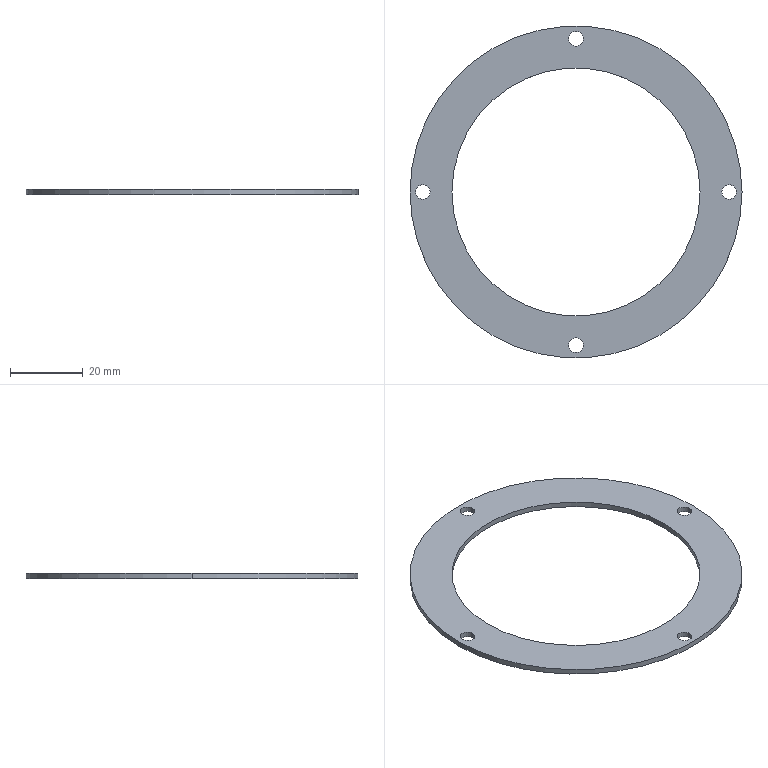Part | STEP file | 31100034--1-S0001 | 1 solid | 14 faces | box 91 x 91 x 1.5 mm | volume 4233 mm3 | cylinder 12 | plane 2 | commonest cylinder face diameters 4 x8 68 x2 91 x2
STEP:
#1=CARTESIAN_POINT('',(0.,0.,0.));
#2=DIRECTION('',(0.,0.,1.));
#3=DIRECTION('',(1.,0.,0.));
#4=AXIS2_PLACEMENT_3D('',#1,#2,#3);
#5=CARTESIAN_POINT('',(-34.,0.,-101.2));
#6=VERTEX_POINT('',#5);
#7=CARTESIAN_POINT('',(-34.,0.,-102.7));
#8=VERTEX_POINT('',#7);
#9=CARTESIAN_POINT('',(-34.,0.,-101.2));
#10=DIRECTION('',(0.,0.,-1.));
#11=VECTOR('',#10,1.);
#12=LINE('',#9,#11);
#13=CARTESIAN_POINT('',(0.,0.,-101.2));
#14=DIRECTION('',(0.,0.,-1.));
#15=DIRECTION('',(-1.,0.,0.));
#16=AXIS2_PLACEMENT_3D('',#13,#14,#15);
#17=CYLINDRICAL_SURFACE('',#16,34.);
#18=CARTESIAN_POINT('',(6.283,0.));
#19=DIRECTION('',(0.,1.));
#20=VECTOR('',#19,1.);
#21=LINE('',#18,#20);
#22=(GEOMETRIC_REPRESENTATION_CONTEXT(2)PARAMETRIC_REPRESENTATION_CONTEXT()REPRESENTATION_CONTEXT('',''));
#23=DEFINITIONAL_REPRESENTATION('',(#21),#22);
#24=PCURVE('',#17,#23);
#25=CARTESIAN_POINT('',(0.,0.,-101.2));
#26=DIRECTION('',(0.,0.,-1.));
#27=DIRECTION('',(-1.,0.,0.));
#28=AXIS2_PLACEMENT_3D('',#25,#26,#27);
#29=CYLINDRICAL_SURFACE('',#28,34.);
#30=CARTESIAN_POINT('',(0.,0.));
#31=DIRECTION('',(0.,1.));
#32=VECTOR('',#31,1.);
#33=LINE('',#30,#32);
#34=(GEOMETRIC_REPRESENTATION_CONTEXT(2)PARAMETRIC_REPRESENTATION_CONTEXT()REPRESENTATION_CONTEXT('',''));
#35=DEFINITIONAL_REPRESENTATION('',(#33),#34);
#36=PCURVE('',#29,#35);
#37=SURFACE_CURVE('',#12,(#24,#36),.PCURVE_S1.);
#38=EDGE_CURVE('',#6,#8,#37,.T.);
#39=ORIENTED_EDGE('',*,*,#38,.T.);
#40=CARTESIAN_POINT('',(34.,0.,-102.7));
#41=VERTEX_POINT('',#40);
#42=CARTESIAN_POINT('',(0.,0.,-102.7));
#43=DIRECTION('',(0.,0.,-1.));
#44=DIRECTION('',(-1.,0.,0.));
#45=AXIS2_PLACEMENT_3D('',#42,#43,#44);
#46=CIRCLE('',#45,34.);
#47=CARTESIAN_POINT('',(0.,1.5));
#48=DIRECTION('',(1.,0.));
#49=VECTOR('',#48,1.);
#50=LINE('',#47,#49);
#51=(GEOMETRIC_REPRESENTATION_CONTEXT(2)PARAMETRIC_REPRESENTATION_CONTEXT()REPRESENTATION_CONTEXT('',''));
#52=DEFINITIONAL_REPRESENTATION('',(#50),#51);
#53=PCURVE('',#17,#52);
#54=CARTESIAN_POINT('',(0.,0.,-102.7));
#55=DIRECTION('',(0.,0.,1.));
#56=DIRECTION('',(1.,0.,0.));
#57=AXIS2_PLACEMENT_3D('',#54,#55,#56);
#58=PLANE('',#57);
#59=CARTESIAN_POINT('',(-34.,0.));
#60=CARTESIAN_POINT('',(-34.,58.89));
#61=CARTESIAN_POINT('',(17.,29.445));
#62=CARTESIAN_POINT('',(68.,0.));
#63=CARTESIAN_POINT('',(17.,-29.445));
#64=CARTESIAN_POINT('',(-34.,-58.89));
#65=CARTESIAN_POINT('',(-34.,0.));
#66=(BOUNDED_CURVE()B_SPLINE_CURVE(2,(#59,#60,#61,#62,#63,#64,#65),.UNSPECIFIED.,.T.,.F.)B_SPLINE_CURVE_WITH_KNOTS((1,2,2,2,2,1),(-2.094,0.,2.094,4.189,6.283,8.378),.UNSPECIFIED.)CURVE()GEOMETRIC_REPRESENTATION_ITEM()RATIONAL_B_SPLINE_CURVE((1.,0.5,1.,0.5,1.,0.5,1.))REPRESENTATION_ITEM(''));
#67=(GEOMETRIC_REPRESENTATION_CONTEXT(2)PARAMETRIC_REPRESENTATION_CONTEXT()REPRESENTATION_CONTEXT('',''));
#68=DEFINITIONAL_REPRESENTATION('',(#66),#67);
#69=PCURVE('',#58,#68);
#70=SURFACE_CURVE('',#46,(#53,#69),.PCURVE_S1.);
#71=EDGE_CURVE('',#41,#8,#70,.T.);
#72=ORIENTED_EDGE('',*,*,#71,.F.);
#73=CARTESIAN_POINT('',(34.,0.,-101.2));
#74=VERTEX_POINT('',#73);
#75=CARTESIAN_POINT('',(34.,0.,-101.2));
#76=DIRECTION('',(0.,0.,-1.));
#77=VECTOR('',#76,1.);
#78=LINE('',#75,#77);
#79=CARTESIAN_POINT('',(3.142,0.));
#80=DIRECTION('',(0.,1.));
#81=VECTOR('',#80,1.);
#82=LINE('',#79,#81);
#83=(GEOMETRIC_REPRESENTATION_CONTEXT(2)PARAMETRIC_REPRESENTATION_CONTEXT()REPRESENTATION_CONTEXT('',''));
#84=DEFINITIONAL_REPRESENTATION('',(#82),#83);
#85=PCURVE('',#17,#84);
#86=CARTESIAN_POINT('',(3.142,0.));
#87=DIRECTION('',(0.,1.));
#88=VECTOR('',#87,1.);
#89=LINE('',#86,#88);
#90=(GEOMETRIC_REPRESENTATION_CONTEXT(2)PARAMETRIC_REPRESENTATION_CONTEXT()REPRESENTATION_CONTEXT('',''));
#91=DEFINITIONAL_REPRESENTATION('',(#89),#90);
#92=PCURVE('',#29,#91);
#93=SURFACE_CURVE('',#78,(#85,#92),.PCURVE_S1.);
#94=EDGE_CURVE('',#74,#41,#93,.T.);
#95=ORIENTED_EDGE('',*,*,#94,.F.);
#96=CARTESIAN_POINT('',(0.,0.,-101.2));
#97=DIRECTION('',(0.,0.,-1.));
#98=DIRECTION('',(-1.,0.,0.));
#99=AXIS2_PLACEMENT_3D('',#96,#97,#98);
#100=CIRCLE('',#99,34.);
#101=CARTESIAN_POINT('',(0.,0.));
#102=DIRECTION('',(1.,0.));
#103=VECTOR('',#102,1.);
#104=LINE('',#101,#103);
#105=(GEOMETRIC_REPRESENTATION_CONTEXT(2)PARAMETRIC_REPRESENTATION_CONTEXT()REPRESENTATION_CONTEXT('',''));
#106=DEFINITIONAL_REPRESENTATION('',(#104),#105);
#107=PCURVE('',#17,#106);
#108=CARTESIAN_POINT('',(0.,0.,-101.2));
#109=DIRECTION('',(0.,0.,1.));
#110=DIRECTION('',(1.,0.,0.));
#111=AXIS2_PLACEMENT_3D('',#108,#109,#110);
#112=PLANE('',#111);
#113=CARTESIAN_POINT('',(-34.,0.));
#114=CARTESIAN_POINT('',(-34.,58.89));
#115=CARTESIAN_POINT('',(17.,29.445));
#116=CARTESIAN_POINT('',(68.,0.));
#117=CARTESIAN_POINT('',(17.,-29.445));
#118=CARTESIAN_POINT('',(-34.,-58.89));
#119=CARTESIAN_POINT('',(-34.,0.));
#120=(BOUNDED_CURVE()B_SPLINE_CURVE(2,(#113,#114,#115,#116,#117,#118,#119),.UNSPECIFIED.,.T.,.F.)B_SPLINE_CURVE_WITH_KNOTS((1,2,2,2,2,1),(-2.094,0.,2.094,4.189,6.283,8.378),.UNSPECIFIED.)CURVE()GEOMETRIC_REPRESENTATION_ITEM()RATIONAL_B_SPLINE_CURVE((1.,0.5,1.,0.5,1.,0.5,1.))REPRESENTATION_ITEM(''));
#121=(GEOMETRIC_REPRESENTATION_CONTEXT(2)PARAMETRIC_REPRESENTATION_CONTEXT()REPRESENTATION_CONTEXT('',''));
#122=DEFINITIONAL_REPRESENTATION('',(#120),#121);
#123=PCURVE('',#112,#122);
#124=SURFACE_CURVE('',#100,(#107,#123),.PCURVE_S1.);
#125=EDGE_CURVE('',#74,#6,#124,.T.);
#126=ORIENTED_EDGE('',*,*,#125,.T.);
#127=EDGE_LOOP('',(#39,#72,#95,#126));
#128=FACE_BOUND('',#127,.F.);
#129=ADVANCED_FACE('',(#128),#17,.F.);
#130=CARTESIAN_POINT('',(44.,0.,-102.7));
#131=VERTEX_POINT('',#130);
#132=CARTESIAN_POINT('',(44.,0.,-101.2));
#133=VERTEX_POINT('',#132);
#134=CARTESIAN_POINT('',(44.,0.,-112.2));
#135=DIRECTION('',(0.,0.,1.));
#136=VECTOR('',#135,1.);
#137=LINE('',#134,#136);
#138=CARTESIAN_POINT('',(42.,0.,-112.2));
#139=DIRECTION('',(0.,0.,1.));
#140=DIRECTION('',(1.,0.,0.));
#141=AXIS2_PLACEMENT_3D('',#138,#139,#140);
#142=CYLINDRICAL_SURFACE('',#141,2.);
#143=CARTESIAN_POINT('',(6.283,0.));
#144=DIRECTION('',(0.,1.));
#145=VECTOR('',#144,1.);
#146=LINE('',#143,#145);
#147=(GEOMETRIC_REPRESENTATION_CONTEXT(2)PARAMETRIC_REPRESENTATION_CONTEXT()REPRESENTATION_CONTEXT('',''));
#148=DEFINITIONAL_REPRESENTATION('',(#146),#147);
#149=PCURVE('',#142,#148);
#150=CARTESIAN_POINT('',(42.,0.,-112.2));
#151=DIRECTION('',(0.,0.,1.));
#152=DIRECTION('',(1.,0.,0.));
#153=AXIS2_PLACEMENT_3D('',#150,#151,#152);
#154=CYLINDRICAL_SURFACE('',#153,2.);
#155=CARTESIAN_POINT('',(0.,0.));
#156=DIRECTION('',(0.,1.));
#157=VECTOR('',#156,1.);
#158=LINE('',#155,#157);
#159=(GEOMETRIC_REPRESENTATION_CONTEXT(2)PARAMETRIC_REPRESENTATION_CONTEXT()REPRESENTATION_CONTEXT('',''));
#160=DEFINITIONAL_REPRESENTATION('',(#158),#159);
#161=PCURVE('',#154,#160);
#162=SURFACE_CURVE('',#137,(#149,#161),.PCURVE_S1.);
#163=EDGE_CURVE('',#131,#133,#162,.T.);
#164=ORIENTED_EDGE('',*,*,#163,.T.);
#165=CARTESIAN_POINT('',(40.,0.,-101.2));
#166=VERTEX_POINT('',#165);
#167=CARTESIAN_POINT('',(42.,0.,-101.2));
#168=DIRECTION('',(0.,0.,-1.));
#169=DIRECTION('',(1.,0.,0.));
#170=AXIS2_PLACEMENT_3D('',#167,#168,#169);
#171=CIRCLE('',#170,2.);
#172=CARTESIAN_POINT('',(6.283,11.));
#173=DIRECTION('',(-1.,0.));
#174=VECTOR('',#173,1.);
#175=LINE('',#172,#174);
#176=(GEOMETRIC_REPRESENTATION_CONTEXT(2)PARAMETRIC_REPRESENTATION_CONTEXT()REPRESENTATION_CONTEXT('',''));
#177=DEFINITIONAL_REPRESENTATION('',(#175),#176);
#178=PCURVE('',#142,#177);
#179=CARTESIAN_POINT('',(44.,0.));
#180=CARTESIAN_POINT('',(44.,-3.464));
#181=CARTESIAN_POINT('',(41.,-1.732));
#182=CARTESIAN_POINT('',(38.,0.));
#183=CARTESIAN_POINT('',(41.,1.732));
#184=CARTESIAN_POINT('',(44.,3.464));
#185=CARTESIAN_POINT('',(44.,0.));
#186=(BOUNDED_CURVE()B_SPLINE_CURVE(2,(#179,#180,#181,#182,#183,#184,#185),.UNSPECIFIED.,.T.,.F.)B_SPLINE_CURVE_WITH_KNOTS((1,2,2,2,2,1),(-2.094,0.,2.094,4.189,6.283,8.378),.UNSPECIFIED.)CURVE()GEOMETRIC_REPRESENTATION_ITEM()RATIONAL_B_SPLINE_CURVE((1.,0.5,1.,0.5,1.,0.5,1.))REPRESENTATION_ITEM(''));
#187=(GEOMETRIC_REPRESENTATION_CONTEXT(2)PARAMETRIC_REPRESENTATION_CONTEXT()REPRESENTATION_CONTEXT('',''));
#188=DEFINITIONAL_REPRESENTATION('',(#186),#187);
#189=PCURVE('',#112,#188);
#190=SURFACE_CURVE('',#171,(#178,#189),.PCURVE_S1.);
#191=EDGE_CURVE('',#133,#166,#190,.T.);
#192=ORIENTED_EDGE('',*,*,#191,.T.);
#193=CARTESIAN_POINT('',(40.,0.,-102.7));
#194=VERTEX_POINT('',#193);
#195=CARTESIAN_POINT('',(40.,0.,-112.2));
#196=DIRECTION('',(0.,0.,1.));
#197=VECTOR('',#196,1.);
#198=LINE('',#195,#197);
#199=CARTESIAN_POINT('',(3.142,0.));
#200=DIRECTION('',(0.,1.));
#201=VECTOR('',#200,1.);
#202=LINE('',#199,#201);
#203=(GEOMETRIC_REPRESENTATION_CONTEXT(2)PARAMETRIC_REPRESENTATION_CONTEXT()REPRESENTATION_CONTEXT('',''));
#204=DEFINITIONAL_REPRESENTATION('',(#202),#203);
#205=PCURVE('',#142,#204);
#206=CARTESIAN_POINT('',(3.142,0.));
#207=DIRECTION('',(0.,1.));
#208=VECTOR('',#207,1.);
#209=LINE('',#206,#208);
#210=(GEOMETRIC_REPRESENTATION_CONTEXT(2)PARAMETRIC_REPRESENTATION_CONTEXT()REPRESENTATION_CONTEXT('',''));
#211=DEFINITIONAL_REPRESENTATION('',(#209),#210);
#212=PCURVE('',#154,#211);
#213=SURFACE_CURVE('',#198,(#205,#212),.PCURVE_S1.);
#214=EDGE_CURVE('',#194,#166,#213,.T.);
#215=ORIENTED_EDGE('',*,*,#214,.F.);
#216=CARTESIAN_POINT('',(42.,0.,-102.7));
#217=DIRECTION('',(0.,0.,-1.));
#218=DIRECTION('',(1.,0.,0.));
#219=AXIS2_PLACEMENT_3D('',#216,#217,#218);
#220=CIRCLE('',#219,2.);
#221=CARTESIAN_POINT('',(6.283,9.5));
#222=DIRECTION('',(-1.,0.));
#223=VECTOR('',#222,1.);
#224=LINE('',#221,#223);
#225=(GEOMETRIC_REPRESENTATION_CONTEXT(2)PARAMETRIC_REPRESENTATION_CONTEXT()REPRESENTATION_CONTEXT('',''));
#226=DEFINITIONAL_REPRESENTATION('',(#224),#225);
#227=PCURVE('',#142,#226);
#228=CARTESIAN_POINT('',(44.,0.));
#229=CARTESIAN_POINT('',(44.,-3.464));
#230=CARTESIAN_POINT('',(41.,-1.732));
#231=CARTESIAN_POINT('',(38.,0.));
#232=CARTESIAN_POINT('',(41.,1.732));
#233=CARTESIAN_POINT('',(44.,3.464));
#234=CARTESIAN_POINT('',(44.,0.));
#235=(BOUNDED_CURVE()B_SPLINE_CURVE(2,(#228,#229,#230,#231,#232,#233,#234),.UNSPECIFIED.,.T.,.F.)B_SPLINE_CURVE_WITH_KNOTS((1,2,2,2,2,1),(-2.094,0.,2.094,4.189,6.283,8.378),.UNSPECIFIED.)CURVE()GEOMETRIC_REPRESENTATION_ITEM()RATIONAL_B_SPLINE_CURVE((1.,0.5,1.,0.5,1.,0.5,1.))REPRESENTATION_ITEM(''));
#236=(GEOMETRIC_REPRESENTATION_CONTEXT(2)PARAMETRIC_REPRESENTATION_CONTEXT()REPRESENTATION_CONTEXT('',''));
#237=DEFINITIONAL_REPRESENTATION('',(#235),#236);
#238=PCURVE('',#58,#237);
#239=SURFACE_CURVE('',#220,(#227,#238),.PCURVE_S1.);
#240=EDGE_CURVE('',#131,#194,#239,.T.);
#241=ORIENTED_EDGE('',*,*,#240,.F.);
#242=EDGE_LOOP('',(#164,#192,#215,#241));
#243=FACE_BOUND('',#242,.F.);
#244=ADVANCED_FACE('',(#243),#142,.F.);
#245=CARTESIAN_POINT('',(2.,-42.,-102.7));
#246=VERTEX_POINT('',#245);
#247=CARTESIAN_POINT('',(2.,-42.,-101.2));
#248=VERTEX_POINT('',#247);
#249=CARTESIAN_POINT('',(2.,-42.,-112.2));
#250=DIRECTION('',(0.,0.,1.));
#251=VECTOR('',#250,1.);
#252=LINE('',#249,#251);
#253=CARTESIAN_POINT('',(0.,-42.,-112.2));
#254=DIRECTION('',(0.,0.,1.));
#255=DIRECTION('',(1.,0.,0.));
#256=AXIS2_PLACEMENT_3D('',#253,#254,#255);
#257=CYLINDRICAL_SURFACE('',#256,2.);
#258=CARTESIAN_POINT('',(6.283,0.));
#259=DIRECTION('',(0.,1.));
#260=VECTOR('',#259,1.);
#261=LINE('',#258,#260);
#262=(GEOMETRIC_REPRESENTATION_CONTEXT(2)PARAMETRIC_REPRESENTATION_CONTEXT()REPRESENTATION_CONTEXT('',''));
#263=DEFINITIONAL_REPRESENTATION('',(#261),#262);
#264=PCURVE('',#257,#263);
#265=CARTESIAN_POINT('',(0.,-42.,-112.2));
#266=DIRECTION('',(0.,0.,1.));
#267=DIRECTION('',(1.,0.,0.));
#268=AXIS2_PLACEMENT_3D('',#265,#266,#267);
#269=CYLINDRICAL_SURFACE('',#268,2.);
#270=CARTESIAN_POINT('',(0.,0.));
#271=DIRECTION('',(0.,1.));
#272=VECTOR('',#271,1.);
#273=LINE('',#270,#272);
#274=(GEOMETRIC_REPRESENTATION_CONTEXT(2)PARAMETRIC_REPRESENTATION_CONTEXT()REPRESENTATION_CONTEXT('',''));
#275=DEFINITIONAL_REPRESENTATION('',(#273),#274);
#276=PCURVE('',#269,#275);
#277=SURFACE_CURVE('',#252,(#264,#276),.PCURVE_S1.);
#278=EDGE_CURVE('',#246,#248,#277,.T.);
#279=ORIENTED_EDGE('',*,*,#278,.T.);
#280=CARTESIAN_POINT('',(-2.,-42.,-101.2));
#281=VERTEX_POINT('',#280);
#282=CARTESIAN_POINT('',(0.,-42.,-101.2));
#283=DIRECTION('',(0.,0.,-1.));
#284=DIRECTION('',(1.,0.,0.));
#285=AXIS2_PLACEMENT_3D('',#282,#283,#284);
#286=CIRCLE('',#285,2.);
#287=CARTESIAN_POINT('',(6.283,11.));
#288=DIRECTION('',(-1.,0.));
#289=VECTOR('',#288,1.);
#290=LINE('',#287,#289);
#291=(GEOMETRIC_REPRESENTATION_CONTEXT(2)PARAMETRIC_REPRESENTATION_CONTEXT()REPRESENTATION_CONTEXT('',''));
#292=DEFINITIONAL_REPRESENTATION('',(#290),#291);
#293=PCURVE('',#257,#292);
#294=CARTESIAN_POINT('',(2.,-42.));
#295=CARTESIAN_POINT('',(2.,-45.464));
#296=CARTESIAN_POINT('',(-1.,-43.732));
#297=CARTESIAN_POINT('',(-4.,-42.));
#298=CARTESIAN_POINT('',(-1.,-40.268));
#299=CARTESIAN_POINT('',(2.,-38.536));
#300=CARTESIAN_POINT('',(2.,-42.));
#301=(BOUNDED_CURVE()B_SPLINE_CURVE(2,(#294,#295,#296,#297,#298,#299,#300),.UNSPECIFIED.,.T.,.F.)B_SPLINE_CURVE_WITH_KNOTS((1,2,2,2,2,1),(-2.094,0.,2.094,4.189,6.283,8.378),.UNSPECIFIED.)CURVE()GEOMETRIC_REPRESENTATION_ITEM()RATIONAL_B_SPLINE_CURVE((1.,0.5,1.,0.5,1.,0.5,1.))REPRESENTATION_ITEM(''));
#302=(GEOMETRIC_REPRESENTATION_CONTEXT(2)PARAMETRIC_REPRESENTATION_CONTEXT()REPRESENTATION_CONTEXT('',''));
#303=DEFINITIONAL_REPRESENTATION('',(#301),#302);
#304=PCURVE('',#112,#303);
#305=SURFACE_CURVE('',#286,(#293,#304),.PCURVE_S1.);
#306=EDGE_CURVE('',#248,#281,#305,.T.);
#307=ORIENTED_EDGE('',*,*,#306,.T.);
#308=CARTESIAN_POINT('',(-2.,-42.,-102.7));
#309=VERTEX_POINT('',#308);
#310=CARTESIAN_POINT('',(-2.,-42.,-112.2));
#311=DIRECTION('',(0.,0.,1.));
#312=VECTOR('',#311,1.);
#313=LINE('',#310,#312);
#314=CARTESIAN_POINT('',(3.142,0.));
#315=DIRECTION('',(0.,1.));
#316=VECTOR('',#315,1.);
#317=LINE('',#314,#316);
#318=(GEOMETRIC_REPRESENTATION_CONTEXT(2)PARAMETRIC_REPRESENTATION_CONTEXT()REPRESENTATION_CONTEXT('',''));
#319=DEFINITIONAL_REPRESENTATION('',(#317),#318);
#320=PCURVE('',#257,#319);
#321=CARTESIAN_POINT('',(3.142,0.));
#322=DIRECTION('',(0.,1.));
#323=VECTOR('',#322,1.);
#324=LINE('',#321,#323);
#325=(GEOMETRIC_REPRESENTATION_CONTEXT(2)PARAMETRIC_REPRESENTATION_CONTEXT()REPRESENTATION_CONTEXT('',''));
#326=DEFINITIONAL_REPRESENTATION('',(#324),#325);
#327=PCURVE('',#269,#326);
#328=SURFACE_CURVE('',#313,(#320,#327),.PCURVE_S1.);
#329=EDGE_CURVE('',#309,#281,#328,.T.);
#330=ORIENTED_EDGE('',*,*,#329,.F.);
#331=CARTESIAN_POINT('',(0.,-42.,-102.7));
#332=DIRECTION('',(0.,0.,-1.));
#333=DIRECTION('',(1.,0.,0.));
#334=AXIS2_PLACEMENT_3D('',#331,#332,#333);
#335=CIRCLE('',#334,2.);
#336=CARTESIAN_POINT('',(6.283,9.5));
#337=DIRECTION('',(-1.,0.));
#338=VECTOR('',#337,1.);
#339=LINE('',#336,#338);
#340=(GEOMETRIC_REPRESENTATION_CONTEXT(2)PARAMETRIC_REPRESENTATION_CONTEXT()REPRESENTATION_CONTEXT('',''));
#341=DEFINITIONAL_REPRESENTATION('',(#339),#340);
#342=PCURVE('',#257,#341);
#343=CARTESIAN_POINT('',(2.,-42.));
#344=CARTESIAN_POINT('',(2.,-45.464));
#345=CARTESIAN_POINT('',(-1.,-43.732));
#346=CARTESIAN_POINT('',(-4.,-42.));
#347=CARTESIAN_POINT('',(-1.,-40.268));
#348=CARTESIAN_POINT('',(2.,-38.536));
#349=CARTESIAN_POINT('',(2.,-42.));
#350=(BOUNDED_CURVE()B_SPLINE_CURVE(2,(#343,#344,#345,#346,#347,#348,#349),.UNSPECIFIED.,.T.,.F.)B_SPLINE_CURVE_WITH_KNOTS((1,2,2,2,2,1),(-2.094,0.,2.094,4.189,6.283,8.378),.UNSPECIFIED.)CURVE()GEOMETRIC_REPRESENTATION_ITEM()RATIONAL_B_SPLINE_CURVE((1.,0.5,1.,0.5,1.,0.5,1.))REPRESENTATION_ITEM(''));
#351=(GEOMETRIC_REPRESENTATION_CONTEXT(2)PARAMETRIC_REPRESENTATION_CONTEXT()REPRESENTATION_CONTEXT('',''));
#352=DEFINITIONAL_REPRESENTATION('',(#350),#351);
#353=PCURVE('',#58,#352);
#354=SURFACE_CURVE('',#335,(#342,#353),.PCURVE_S1.);
#355=EDGE_CURVE('',#246,#309,#354,.T.);
#356=ORIENTED_EDGE('',*,*,#355,.F.);
#357=EDGE_LOOP('',(#279,#307,#330,#356));
#358=FACE_BOUND('',#357,.F.);
#359=ADVANCED_FACE('',(#358),#257,.F.);
#360=CARTESIAN_POINT('',(-40.,0.,-102.7));
#361=VERTEX_POINT('',#360);
#362=CARTESIAN_POINT('',(-40.,0.,-101.2));
#363=VERTEX_POINT('',#362);
#364=CARTESIAN_POINT('',(-40.,0.,-112.2));
#365=DIRECTION('',(0.,0.,1.));
#366=VECTOR('',#365,1.);
#367=LINE('',#364,#366);
#368=CARTESIAN_POINT('',(-42.,0.,-112.2));
#369=DIRECTION('',(0.,0.,1.));
#370=DIRECTION('',(1.,0.,0.));
#371=AXIS2_PLACEMENT_3D('',#368,#369,#370);
#372=CYLINDRICAL_SURFACE('',#371,2.);
#373=CARTESIAN_POINT('',(6.283,0.));
#374=DIRECTION('',(0.,1.));
#375=VECTOR('',#374,1.);
#376=LINE('',#373,#375);
#377=(GEOMETRIC_REPRESENTATION_CONTEXT(2)PARAMETRIC_REPRESENTATION_CONTEXT()REPRESENTATION_CONTEXT('',''));
#378=DEFINITIONAL_REPRESENTATION('',(#376),#377);
#379=PCURVE('',#372,#378);
#380=CARTESIAN_POINT('',(-42.,0.,-112.2));
#381=DIRECTION('',(0.,0.,1.));
#382=DIRECTION('',(1.,0.,0.));
#383=AXIS2_PLACEMENT_3D('',#380,#381,#382);
#384=CYLINDRICAL_SURFACE('',#383,2.);
#385=CARTESIAN_POINT('',(0.,0.));
#386=DIRECTION('',(0.,1.));
#387=VECTOR('',#386,1.);
#388=LINE('',#385,#387);
#389=(GEOMETRIC_REPRESENTATION_CONTEXT(2)PARAMETRIC_REPRESENTATION_CONTEXT()REPRESENTATION_CONTEXT('',''));
#390=DEFINITIONAL_REPRESENTATION('',(#388),#389);
#391=PCURVE('',#384,#390);
#392=SURFACE_CURVE('',#367,(#379,#391),.PCURVE_S1.);
#393=EDGE_CURVE('',#361,#363,#392,.T.);
#394=ORIENTED_EDGE('',*,*,#393,.T.);
#395=CARTESIAN_POINT('',(-44.,0.,-101.2));
#396=VERTEX_POINT('',#395);
#397=CARTESIAN_POINT('',(-42.,0.,-101.2));
#398=DIRECTION('',(0.,0.,-1.));
#399=DIRECTION('',(1.,0.,0.));
#400=AXIS2_PLACEMENT_3D('',#397,#398,#399);
#401=CIRCLE('',#400,2.);
#402=CARTESIAN_POINT('',(6.283,11.));
#403=DIRECTION('',(-1.,0.));
#404=VECTOR('',#403,1.);
#405=LINE('',#402,#404);
#406=(GEOMETRIC_REPRESENTATION_CONTEXT(2)PARAMETRIC_REPRESENTATION_CONTEXT()REPRESENTATION_CONTEXT('',''));
#407=DEFINITIONAL_REPRESENTATION('',(#405),#406);
#408=PCURVE('',#372,#407);
#409=CARTESIAN_POINT('',(-40.,0.));
#410=CARTESIAN_POINT('',(-40.,-3.464));
#411=CARTESIAN_POINT('',(-43.,-1.732));
#412=CARTESIAN_POINT('',(-46.,0.));
#413=CARTESIAN_POINT('',(-43.,1.732));
#414=CARTESIAN_POINT('',(-40.,3.464));
#415=CARTESIAN_POINT('',(-40.,0.));
#416=(BOUNDED_CURVE()B_SPLINE_CURVE(2,(#409,#410,#411,#412,#413,#414,#415),.UNSPECIFIED.,.T.,.F.)B_SPLINE_CURVE_WITH_KNOTS((1,2,2,2,2,1),(-2.094,0.,2.094,4.189,6.283,8.378),.UNSPECIFIED.)CURVE()GEOMETRIC_REPRESENTATION_ITEM()RATIONAL_B_SPLINE_CURVE((1.,0.5,1.,0.5,1.,0.5,1.))REPRESENTATION_ITEM(''));
#417=(GEOMETRIC_REPRESENTATION_CONTEXT(2)PARAMETRIC_REPRESENTATION_CONTEXT()REPRESENTATION_CONTEXT('',''));
#418=DEFINITIONAL_REPRESENTATION('',(#416),#417);
#419=PCURVE('',#112,#418);
#420=SURFACE_CURVE('',#401,(#408,#419),.PCURVE_S1.);
#421=EDGE_CURVE('',#363,#396,#420,.T.);
#422=ORIENTED_EDGE('',*,*,#421,.T.);
#423=CARTESIAN_POINT('',(-44.,0.,-102.7));
#424=VERTEX_POINT('',#423);
#425=CARTESIAN_POINT('',(-44.,0.,-112.2));
#426=DIRECTION('',(0.,0.,1.));
#427=VECTOR('',#426,1.);
#428=LINE('',#425,#427);
#429=CARTESIAN_POINT('',(3.142,0.));
#430=DIRECTION('',(0.,1.));
#431=VECTOR('',#430,1.);
#432=LINE('',#429,#431);
#433=(GEOMETRIC_REPRESENTATION_CONTEXT(2)PARAMETRIC_REPRESENTATION_CONTEXT()REPRESENTATION_CONTEXT('',''));
#434=DEFINITIONAL_REPRESENTATION('',(#432),#433);
#435=PCURVE('',#372,#434);
#436=CARTESIAN_POINT('',(3.142,0.));
#437=DIRECTION('',(0.,1.));
#438=VECTOR('',#437,1.);
#439=LINE('',#436,#438);
#440=(GEOMETRIC_REPRESENTATION_CONTEXT(2)PARAMETRIC_REPRESENTATION_CONTEXT()REPRESENTATION_CONTEXT('',''));
#441=DEFINITIONAL_REPRESENTATION('',(#439),#440);
#442=PCURVE('',#384,#441);
#443=SURFACE_CURVE('',#428,(#435,#442),.PCURVE_S1.);
#444=EDGE_CURVE('',#424,#396,#443,.T.);
#445=ORIENTED_EDGE('',*,*,#444,.F.);
#446=CARTESIAN_POINT('',(-42.,0.,-102.7));
#447=DIRECTION('',(0.,0.,-1.));
#448=DIRECTION('',(1.,0.,0.));
#449=AXIS2_PLACEMENT_3D('',#446,#447,#448);
#450=CIRCLE('',#449,2.);
#451=CARTESIAN_POINT('',(6.283,9.5));
#452=DIRECTION('',(-1.,0.));
#453=VECTOR('',#452,1.);
#454=LINE('',#451,#453);
#455=(GEOMETRIC_REPRESENTATION_CONTEXT(2)PARAMETRIC_REPRESENTATION_CONTEXT()REPRESENTATION_CONTEXT('',''));
#456=DEFINITIONAL_REPRESENTATION('',(#454),#455);
#457=PCURVE('',#372,#456);
#458=CARTESIAN_POINT('',(-40.,0.));
#459=CARTESIAN_POINT('',(-40.,-3.464));
#460=CARTESIAN_POINT('',(-43.,-1.732));
#461=CARTESIAN_POINT('',(-46.,0.));
#462=CARTESIAN_POINT('',(-43.,1.732));
#463=CARTESIAN_POINT('',(-40.,3.464));
#464=CARTESIAN_POINT('',(-40.,0.));
#465=(BOUNDED_CURVE()B_SPLINE_CURVE(2,(#458,#459,#460,#461,#462,#463,#464),.UNSPECIFIED.,.T.,.F.)B_SPLINE_CURVE_WITH_KNOTS((1,2,2,2,2,1),(-2.094,0.,2.094,4.189,6.283,8.378),.UNSPECIFIED.)CURVE()GEOMETRIC_REPRESENTATION_ITEM()RATIONAL_B_SPLINE_CURVE((1.,0.5,1.,0.5,1.,0.5,1.))REPRESENTATION_ITEM(''));
#466=(GEOMETRIC_REPRESENTATION_CONTEXT(2)PARAMETRIC_REPRESENTATION_CONTEXT()REPRESENTATION_CONTEXT('',''));
#467=DEFINITIONAL_REPRESENTATION('',(#465),#466);
#468=PCURVE('',#58,#467);
#469=SURFACE_CURVE('',#450,(#457,#468),.PCURVE_S1.);
#470=EDGE_CURVE('',#361,#424,#469,.T.);
#471=ORIENTED_EDGE('',*,*,#470,.F.);
#472=EDGE_LOOP('',(#394,#422,#445,#471));
#473=FACE_BOUND('',#472,.F.);
#474=ADVANCED_FACE('',(#473),#372,.F.);
#475=CARTESIAN_POINT('',(2.,42.,-102.7));
#476=VERTEX_POINT('',#475);
#477=CARTESIAN_POINT('',(2.,42.,-101.2));
#478=VERTEX_POINT('',#477);
#479=CARTESIAN_POINT('',(2.,42.,-112.2));
#480=DIRECTION('',(0.,0.,1.));
#481=VECTOR('',#480,1.);
#482=LINE('',#479,#481);
#483=CARTESIAN_POINT('',(0.,42.,-112.2));
#484=DIRECTION('',(0.,0.,1.));
#485=DIRECTION('',(1.,0.,0.));
#486=AXIS2_PLACEMENT_3D('',#483,#484,#485);
#487=CYLINDRICAL_SURFACE('',#486,2.);
#488=CARTESIAN_POINT('',(6.283,0.));
#489=DIRECTION('',(0.,1.));
#490=VECTOR('',#489,1.);
#491=LINE('',#488,#490);
#492=(GEOMETRIC_REPRESENTATION_CONTEXT(2)PARAMETRIC_REPRESENTATION_CONTEXT()REPRESENTATION_CONTEXT('',''));
#493=DEFINITIONAL_REPRESENTATION('',(#491),#492);
#494=PCURVE('',#487,#493);
#495=CARTESIAN_POINT('',(0.,42.,-112.2));
#496=DIRECTION('',(0.,0.,1.));
#497=DIRECTION('',(1.,0.,0.));
#498=AXIS2_PLACEMENT_3D('',#495,#496,#497);
#499=CYLINDRICAL_SURFACE('',#498,2.);
#500=CARTESIAN_POINT('',(0.,0.));
#501=DIRECTION('',(0.,1.));
#502=VECTOR('',#501,1.);
#503=LINE('',#500,#502);
#504=(GEOMETRIC_REPRESENTATION_CONTEXT(2)PARAMETRIC_REPRESENTATION_CONTEXT()REPRESENTATION_CONTEXT('',''));
#505=DEFINITIONAL_REPRESENTATION('',(#503),#504);
#506=PCURVE('',#499,#505);
#507=SURFACE_CURVE('',#482,(#494,#506),.PCURVE_S1.);
#508=EDGE_CURVE('',#476,#478,#507,.T.);
#509=ORIENTED_EDGE('',*,*,#508,.T.);
#510=CARTESIAN_POINT('',(-2.,42.,-101.2));
#511=VERTEX_POINT('',#510);
#512=CARTESIAN_POINT('',(0.,42.,-101.2));
#513=DIRECTION('',(0.,0.,-1.));
#514=DIRECTION('',(1.,0.,0.));
#515=AXIS2_PLACEMENT_3D('',#512,#513,#514);
#516=CIRCLE('',#515,2.);
#517=CARTESIAN_POINT('',(6.283,11.));
#518=DIRECTION('',(-1.,0.));
#519=VECTOR('',#518,1.);
#520=LINE('',#517,#519);
#521=(GEOMETRIC_REPRESENTATION_CONTEXT(2)PARAMETRIC_REPRESENTATION_CONTEXT()REPRESENTATION_CONTEXT('',''));
#522=DEFINITIONAL_REPRESENTATION('',(#520),#521);
#523=PCURVE('',#487,#522);
#524=CARTESIAN_POINT('',(2.,42.));
#525=CARTESIAN_POINT('',(2.,38.536));
#526=CARTESIAN_POINT('',(-1.,40.268));
#527=CARTESIAN_POINT('',(-4.,42.));
#528=CARTESIAN_POINT('',(-1.,43.732));
#529=CARTESIAN_POINT('',(2.,45.464));
#530=CARTESIAN_POINT('',(2.,42.));
#531=(BOUNDED_CURVE()B_SPLINE_CURVE(2,(#524,#525,#526,#527,#528,#529,#530),.UNSPECIFIED.,.T.,.F.)B_SPLINE_CURVE_WITH_KNOTS((1,2,2,2,2,1),(-2.094,0.,2.094,4.189,6.283,8.378),.UNSPECIFIED.)CURVE()GEOMETRIC_REPRESENTATION_ITEM()RATIONAL_B_SPLINE_CURVE((1.,0.5,1.,0.5,1.,0.5,1.))REPRESENTATION_ITEM(''));
#532=(GEOMETRIC_REPRESENTATION_CONTEXT(2)PARAMETRIC_REPRESENTATION_CONTEXT()REPRESENTATION_CONTEXT('',''));
#533=DEFINITIONAL_REPRESENTATION('',(#531),#532);
#534=PCURVE('',#112,#533);
#535=SURFACE_CURVE('',#516,(#523,#534),.PCURVE_S1.);
#536=EDGE_CURVE('',#478,#511,#535,.T.);
#537=ORIENTED_EDGE('',*,*,#536,.T.);
#538=CARTESIAN_POINT('',(-2.,42.,-102.7));
#539=VERTEX_POINT('',#538);
#540=CARTESIAN_POINT('',(-2.,42.,-112.2));
#541=DIRECTION('',(0.,0.,1.));
#542=VECTOR('',#541,1.);
#543=LINE('',#540,#542);
#544=CARTESIAN_POINT('',(3.142,0.));
#545=DIRECTION('',(0.,1.));
#546=VECTOR('',#545,1.);
#547=LINE('',#544,#546);
#548=(GEOMETRIC_REPRESENTATION_CONTEXT(2)PARAMETRIC_REPRESENTATION_CONTEXT()REPRESENTATION_CONTEXT('',''));
#549=DEFINITIONAL_REPRESENTATION('',(#547),#548);
#550=PCURVE('',#487,#549);
#551=CARTESIAN_POINT('',(3.142,0.));
#552=DIRECTION('',(0.,1.));
#553=VECTOR('',#552,1.);
#554=LINE('',#551,#553);
#555=(GEOMETRIC_REPRESENTATION_CONTEXT(2)PARAMETRIC_REPRESENTATION_CONTEXT()REPRESENTATION_CONTEXT('',''));
#556=DEFINITIONAL_REPRESENTATION('',(#554),#555);
#557=PCURVE('',#499,#556);
#558=SURFACE_CURVE('',#543,(#550,#557),.PCURVE_S1.);
#559=EDGE_CURVE('',#539,#511,#558,.T.);
#560=ORIENTED_EDGE('',*,*,#559,.F.);
#561=CARTESIAN_POINT('',(0.,42.,-102.7));
#562=DIRECTION('',(0.,0.,-1.));
#563=DIRECTION('',(1.,0.,0.));
#564=AXIS2_PLACEMENT_3D('',#561,#562,#563);
#565=CIRCLE('',#564,2.);
#566=CARTESIAN_POINT('',(6.283,9.5));
#567=DIRECTION('',(-1.,0.));
#568=VECTOR('',#567,1.);
#569=LINE('',#566,#568);
#570=(GEOMETRIC_REPRESENTATION_CONTEXT(2)PARAMETRIC_REPRESENTATION_CONTEXT()REPRESENTATION_CONTEXT('',''));
#571=DEFINITIONAL_REPRESENTATION('',(#569),#570);
#572=PCURVE('',#487,#571);
#573=CARTESIAN_POINT('',(2.,42.));
#574=CARTESIAN_POINT('',(2.,38.536));
#575=CARTESIAN_POINT('',(-1.,40.268));
#576=CARTESIAN_POINT('',(-4.,42.));
#577=CARTESIAN_POINT('',(-1.,43.732));
#578=CARTESIAN_POINT('',(2.,45.464));
#579=CARTESIAN_POINT('',(2.,42.));
#580=(BOUNDED_CURVE()B_SPLINE_CURVE(2,(#573,#574,#575,#576,#577,#578,#579),.UNSPECIFIED.,.T.,.F.)B_SPLINE_CURVE_WITH_KNOTS((1,2,2,2,2,1),(-2.094,0.,2.094,4.189,6.283,8.378),.UNSPECIFIED.)CURVE()GEOMETRIC_REPRESENTATION_ITEM()RATIONAL_B_SPLINE_CURVE((1.,0.5,1.,0.5,1.,0.5,1.))REPRESENTATION_ITEM(''));
#581=(GEOMETRIC_REPRESENTATION_CONTEXT(2)PARAMETRIC_REPRESENTATION_CONTEXT()REPRESENTATION_CONTEXT('',''));
#582=DEFINITIONAL_REPRESENTATION('',(#580),#581);
#583=PCURVE('',#58,#582);
#584=SURFACE_CURVE('',#565,(#572,#583),.PCURVE_S1.);
#585=EDGE_CURVE('',#476,#539,#584,.T.);
#586=ORIENTED_EDGE('',*,*,#585,.F.);
#587=EDGE_LOOP('',(#509,#537,#560,#586));
#588=FACE_BOUND('',#587,.F.);
#589=ADVANCED_FACE('',(#588),#487,.F.);
#590=CARTESIAN_POINT('',(-45.5,0.,-101.2));
#591=VERTEX_POINT('',#590);
#592=CARTESIAN_POINT('',(45.5,0.,-101.2));
#593=VERTEX_POINT('',#592);
#594=CARTESIAN_POINT('',(0.,0.,-101.2));
#595=DIRECTION('',(0.,0.,-1.));
#596=DIRECTION('',(-1.,0.,0.));
#597=AXIS2_PLACEMENT_3D('',#594,#595,#596);
#598=CIRCLE('',#597,45.5);
#599=CARTESIAN_POINT('',(0.,0.,-101.2));
#600=DIRECTION('',(0.,0.,-1.));
#601=DIRECTION('',(-1.,0.,0.));
#602=AXIS2_PLACEMENT_3D('',#599,#600,#601);
#603=CYLINDRICAL_SURFACE('',#602,45.5);
#604=CARTESIAN_POINT('',(0.,0.));
#605=DIRECTION('',(1.,0.));
#606=VECTOR('',#605,1.);
#607=LINE('',#604,#606);
#608=(GEOMETRIC_REPRESENTATION_CONTEXT(2)PARAMETRIC_REPRESENTATION_CONTEXT()REPRESENTATION_CONTEXT('',''));
#609=DEFINITIONAL_REPRESENTATION('',(#607),#608);
#610=PCURVE('',#603,#609);
#611=CARTESIAN_POINT('',(-45.5,0.));
#612=CARTESIAN_POINT('',(-45.5,78.808));
#613=CARTESIAN_POINT('',(22.75,39.404));
#614=CARTESIAN_POINT('',(91.,0.));
#615=CARTESIAN_POINT('',(22.75,-39.404));
#616=CARTESIAN_POINT('',(-45.5,-78.808));
#617=CARTESIAN_POINT('',(-45.5,0.));
#618=(BOUNDED_CURVE()B_SPLINE_CURVE(2,(#611,#612,#613,#614,#615,#616,#617),.UNSPECIFIED.,.T.,.F.)B_SPLINE_CURVE_WITH_KNOTS((1,2,2,2,2,1),(-2.094,0.,2.094,4.189,6.283,8.378),.UNSPECIFIED.)CURVE()GEOMETRIC_REPRESENTATION_ITEM()RATIONAL_B_SPLINE_CURVE((1.,0.5,1.,0.5,1.,0.5,1.))REPRESENTATION_ITEM(''));
#619=(GEOMETRIC_REPRESENTATION_CONTEXT(2)PARAMETRIC_REPRESENTATION_CONTEXT()REPRESENTATION_CONTEXT('',''));
#620=DEFINITIONAL_REPRESENTATION('',(#618),#619);
#621=PCURVE('',#112,#620);
#622=SURFACE_CURVE('',#598,(#610,#621),.PCURVE_S1.);
#623=EDGE_CURVE('',#591,#593,#622,.T.);
#624=ORIENTED_EDGE('',*,*,#623,.T.);
#625=CARTESIAN_POINT('',(45.5,0.,-102.7));
#626=VERTEX_POINT('',#625);
#627=CARTESIAN_POINT('',(45.5,0.,-101.2));
#628=DIRECTION('',(0.,0.,-1.));
#629=VECTOR('',#628,1.);
#630=LINE('',#627,#629);
#631=CARTESIAN_POINT('',(3.142,0.));
#632=DIRECTION('',(0.,1.));
#633=VECTOR('',#632,1.);
#634=LINE('',#631,#633);
#635=(GEOMETRIC_REPRESENTATION_CONTEXT(2)PARAMETRIC_REPRESENTATION_CONTEXT()REPRESENTATION_CONTEXT('',''));
#636=DEFINITIONAL_REPRESENTATION('',(#634),#635);
#637=PCURVE('',#603,#636);
#638=CARTESIAN_POINT('',(0.,0.,-101.2));
#639=DIRECTION('',(0.,0.,-1.));
#640=DIRECTION('',(-1.,0.,0.));
#641=AXIS2_PLACEMENT_3D('',#638,#639,#640);
#642=CYLINDRICAL_SURFACE('',#641,45.5);
#643=CARTESIAN_POINT('',(3.142,0.));
#644=DIRECTION('',(0.,1.));
#645=VECTOR('',#644,1.);
#646=LINE('',#643,#645);
#647=(GEOMETRIC_REPRESENTATION_CONTEXT(2)PARAMETRIC_REPRESENTATION_CONTEXT()REPRESENTATION_CONTEXT('',''));
#648=DEFINITIONAL_REPRESENTATION('',(#646),#647);
#649=PCURVE('',#642,#648);
#650=SURFACE_CURVE('',#630,(#637,#649),.PCURVE_S1.);
#651=EDGE_CURVE('',#593,#626,#650,.T.);
#652=ORIENTED_EDGE('',*,*,#651,.T.);
#653=CARTESIAN_POINT('',(-45.5,0.,-102.7));
#654=VERTEX_POINT('',#653);
#655=CARTESIAN_POINT('',(0.,0.,-102.7));
#656=DIRECTION('',(0.,0.,1.));
#657=DIRECTION('',(-1.,0.,0.));
#658=AXIS2_PLACEMENT_3D('',#655,#656,#657);
#659=CIRCLE('',#658,45.5);
#660=CARTESIAN_POINT('',(6.283,1.5));
#661=DIRECTION('',(-1.,0.));
#662=VECTOR('',#661,1.);
#663=LINE('',#660,#662);
#664=(GEOMETRIC_REPRESENTATION_CONTEXT(2)PARAMETRIC_REPRESENTATION_CONTEXT()REPRESENTATION_CONTEXT('',''));
#665=DEFINITIONAL_REPRESENTATION('',(#663),#664);
#666=PCURVE('',#603,#665);
#667=CARTESIAN_POINT('',(0.,0.));
#668=DIRECTION('',(-1.,0.));
#669=AXIS2_PLACEMENT_2D('',#667,#668);
#670=CIRCLE('',#669,45.5);
#671=(GEOMETRIC_REPRESENTATION_CONTEXT(2)PARAMETRIC_REPRESENTATION_CONTEXT()REPRESENTATION_CONTEXT('',''));
#672=DEFINITIONAL_REPRESENTATION('',(#670),#671);
#673=PCURVE('',#58,#672);
#674=SURFACE_CURVE('',#659,(#666,#673),.PCURVE_S1.);
#675=EDGE_CURVE('',#626,#654,#674,.T.);
#676=ORIENTED_EDGE('',*,*,#675,.T.);
#677=CARTESIAN_POINT('',(-45.5,0.,-101.2));
#678=DIRECTION('',(0.,0.,-1.));
#679=VECTOR('',#678,1.);
#680=LINE('',#677,#679);
#681=CARTESIAN_POINT('',(0.,0.));
#682=DIRECTION('',(0.,1.));
#683=VECTOR('',#682,1.);
#684=LINE('',#681,#683);
#685=(GEOMETRIC_REPRESENTATION_CONTEXT(2)PARAMETRIC_REPRESENTATION_CONTEXT()REPRESENTATION_CONTEXT('',''));
#686=DEFINITIONAL_REPRESENTATION('',(#684),#685);
#687=PCURVE('',#603,#686);
#688=CARTESIAN_POINT('',(6.283,0.));
#689=DIRECTION('',(0.,1.));
#690=VECTOR('',#689,1.);
#691=LINE('',#688,#690);
#692=(GEOMETRIC_REPRESENTATION_CONTEXT(2)PARAMETRIC_REPRESENTATION_CONTEXT()REPRESENTATION_CONTEXT('',''));
#693=DEFINITIONAL_REPRESENTATION('',(#691),#692);
#694=PCURVE('',#642,#693);
#695=SURFACE_CURVE('',#680,(#687,#694),.PCURVE_S1.);
#696=EDGE_CURVE('',#591,#654,#695,.T.);
#697=ORIENTED_EDGE('',*,*,#696,.F.);
#698=EDGE_LOOP('',(#624,#652,#676,#697));
#699=FACE_BOUND('',#698,.T.);
#700=ADVANCED_FACE('',(#699),#603,.T.);
#701=CARTESIAN_POINT('',(0.,0.,-102.7));
#702=DIRECTION('',(0.,0.,-1.));
#703=DIRECTION('',(-1.,0.,0.));
#704=AXIS2_PLACEMENT_3D('',#701,#702,#703);
#705=CIRCLE('',#704,34.);
#706=CARTESIAN_POINT('',(-34.,0.));
#707=CARTESIAN_POINT('',(-34.,58.89));
#708=CARTESIAN_POINT('',(17.,29.445));
#709=CARTESIAN_POINT('',(68.,0.));
#710=CARTESIAN_POINT('',(17.,-29.445));
#711=CARTESIAN_POINT('',(-34.,-58.89));
#712=CARTESIAN_POINT('',(-34.,0.));
#713=(BOUNDED_CURVE()B_SPLINE_CURVE(2,(#706,#707,#708,#709,#710,#711,#712),.UNSPECIFIED.,.T.,.F.)B_SPLINE_CURVE_WITH_KNOTS((1,2,2,2,2,1),(-2.094,0.,2.094,4.189,6.283,8.378),.UNSPECIFIED.)CURVE()GEOMETRIC_REPRESENTATION_ITEM()RATIONAL_B_SPLINE_CURVE((1.,0.5,1.,0.5,1.,0.5,1.))REPRESENTATION_ITEM(''));
#714=(GEOMETRIC_REPRESENTATION_CONTEXT(2)PARAMETRIC_REPRESENTATION_CONTEXT()REPRESENTATION_CONTEXT('',''));
#715=DEFINITIONAL_REPRESENTATION('',(#713),#714);
#716=PCURVE('',#58,#715);
#717=CARTESIAN_POINT('',(0.,1.5));
#718=DIRECTION('',(1.,0.));
#719=VECTOR('',#718,1.);
#720=LINE('',#717,#719);
#721=(GEOMETRIC_REPRESENTATION_CONTEXT(2)PARAMETRIC_REPRESENTATION_CONTEXT()REPRESENTATION_CONTEXT('',''));
#722=DEFINITIONAL_REPRESENTATION('',(#720),#721);
#723=PCURVE('',#29,#722);
#724=SURFACE_CURVE('',#705,(#716,#723),.PCURVE_S1.);
#725=EDGE_CURVE('',#8,#41,#724,.T.);
#726=ORIENTED_EDGE('',*,*,#725,.F.);
#727=ORIENTED_EDGE('',*,*,#71,.F.);
#728=EDGE_LOOP('',(#726,#727));
#729=FACE_BOUND('',#728,.T.);
#730=ORIENTED_EDGE('',*,*,#240,.F.);
#731=CARTESIAN_POINT('',(42.,0.,-102.7));
#732=DIRECTION('',(0.,0.,-1.));
#733=DIRECTION('',(1.,0.,0.));
#734=AXIS2_PLACEMENT_3D('',#731,#732,#733);
#735=CIRCLE('',#734,2.);
#736=CARTESIAN_POINT('',(44.,0.));
#737=CARTESIAN_POINT('',(44.,-3.464));
#738=CARTESIAN_POINT('',(41.,-1.732));
#739=CARTESIAN_POINT('',(38.,0.));
#740=CARTESIAN_POINT('',(41.,1.732));
#741=CARTESIAN_POINT('',(44.,3.464));
#742=CARTESIAN_POINT('',(44.,0.));
#743=(BOUNDED_CURVE()B_SPLINE_CURVE(2,(#736,#737,#738,#739,#740,#741,#742),.UNSPECIFIED.,.T.,.F.)B_SPLINE_CURVE_WITH_KNOTS((1,2,2,2,2,1),(-2.094,0.,2.094,4.189,6.283,8.378),.UNSPECIFIED.)CURVE()GEOMETRIC_REPRESENTATION_ITEM()RATIONAL_B_SPLINE_CURVE((1.,0.5,1.,0.5,1.,0.5,1.))REPRESENTATION_ITEM(''));
#744=(GEOMETRIC_REPRESENTATION_CONTEXT(2)PARAMETRIC_REPRESENTATION_CONTEXT()REPRESENTATION_CONTEXT('',''));
#745=DEFINITIONAL_REPRESENTATION('',(#743),#744);
#746=PCURVE('',#58,#745);
#747=CARTESIAN_POINT('',(6.283,9.5));
#748=DIRECTION('',(-1.,0.));
#749=VECTOR('',#748,1.);
#750=LINE('',#747,#749);
#751=(GEOMETRIC_REPRESENTATION_CONTEXT(2)PARAMETRIC_REPRESENTATION_CONTEXT()REPRESENTATION_CONTEXT('',''));
#752=DEFINITIONAL_REPRESENTATION('',(#750),#751);
#753=PCURVE('',#154,#752);
#754=SURFACE_CURVE('',#735,(#746,#753),.PCURVE_S1.);
#755=EDGE_CURVE('',#194,#131,#754,.T.);
#756=ORIENTED_EDGE('',*,*,#755,.F.);
#757=EDGE_LOOP('',(#730,#756));
#758=FACE_BOUND('',#757,.T.);
#759=ORIENTED_EDGE('',*,*,#355,.F.);
#760=CARTESIAN_POINT('',(0.,-42.,-102.7));
#761=DIRECTION('',(0.,0.,-1.));
#762=DIRECTION('',(1.,0.,0.));
#763=AXIS2_PLACEMENT_3D('',#760,#761,#762);
#764=CIRCLE('',#763,2.);
#765=CARTESIAN_POINT('',(2.,-42.));
#766=CARTESIAN_POINT('',(2.,-45.464));
#767=CARTESIAN_POINT('',(-1.,-43.732));
#768=CARTESIAN_POINT('',(-4.,-42.));
#769=CARTESIAN_POINT('',(-1.,-40.268));
#770=CARTESIAN_POINT('',(2.,-38.536));
#771=CARTESIAN_POINT('',(2.,-42.));
#772=(BOUNDED_CURVE()B_SPLINE_CURVE(2,(#765,#766,#767,#768,#769,#770,#771),.UNSPECIFIED.,.T.,.F.)B_SPLINE_CURVE_WITH_KNOTS((1,2,2,2,2,1),(-2.094,0.,2.094,4.189,6.283,8.378),.UNSPECIFIED.)CURVE()GEOMETRIC_REPRESENTATION_ITEM()RATIONAL_B_SPLINE_CURVE((1.,0.5,1.,0.5,1.,0.5,1.))REPRESENTATION_ITEM(''));
#773=(GEOMETRIC_REPRESENTATION_CONTEXT(2)PARAMETRIC_REPRESENTATION_CONTEXT()REPRESENTATION_CONTEXT('',''));
#774=DEFINITIONAL_REPRESENTATION('',(#772),#773);
#775=PCURVE('',#58,#774);
#776=CARTESIAN_POINT('',(6.283,9.5));
#777=DIRECTION('',(-1.,0.));
#778=VECTOR('',#777,1.);
#779=LINE('',#776,#778);
#780=(GEOMETRIC_REPRESENTATION_CONTEXT(2)PARAMETRIC_REPRESENTATION_CONTEXT()REPRESENTATION_CONTEXT('',''));
#781=DEFINITIONAL_REPRESENTATION('',(#779),#780);
#782=PCURVE('',#269,#781);
#783=SURFACE_CURVE('',#764,(#775,#782),.PCURVE_S1.);
#784=EDGE_CURVE('',#309,#246,#783,.T.);
#785=ORIENTED_EDGE('',*,*,#784,.F.);
#786=EDGE_LOOP('',(#759,#785));
#787=FACE_BOUND('',#786,.T.);
#788=ORIENTED_EDGE('',*,*,#470,.F.);
#789=CARTESIAN_POINT('',(-42.,0.,-102.7));
#790=DIRECTION('',(0.,0.,-1.));
#791=DIRECTION('',(1.,0.,0.));
#792=AXIS2_PLACEMENT_3D('',#789,#790,#791);
#793=CIRCLE('',#792,2.);
#794=CARTESIAN_POINT('',(-40.,0.));
#795=CARTESIAN_POINT('',(-40.,-3.464));
#796=CARTESIAN_POINT('',(-43.,-1.732));
#797=CARTESIAN_POINT('',(-46.,0.));
#798=CARTESIAN_POINT('',(-43.,1.732));
#799=CARTESIAN_POINT('',(-40.,3.464));
#800=CARTESIAN_POINT('',(-40.,0.));
#801=(BOUNDED_CURVE()B_SPLINE_CURVE(2,(#794,#795,#796,#797,#798,#799,#800),.UNSPECIFIED.,.T.,.F.)B_SPLINE_CURVE_WITH_KNOTS((1,2,2,2,2,1),(-2.094,0.,2.094,4.189,6.283,8.378),.UNSPECIFIED.)CURVE()GEOMETRIC_REPRESENTATION_ITEM()RATIONAL_B_SPLINE_CURVE((1.,0.5,1.,0.5,1.,0.5,1.))REPRESENTATION_ITEM(''));
#802=(GEOMETRIC_REPRESENTATION_CONTEXT(2)PARAMETRIC_REPRESENTATION_CONTEXT()REPRESENTATION_CONTEXT('',''));
#803=DEFINITIONAL_REPRESENTATION('',(#801),#802);
#804=PCURVE('',#58,#803);
#805=CARTESIAN_POINT('',(6.283,9.5));
#806=DIRECTION('',(-1.,0.));
#807=VECTOR('',#806,1.);
#808=LINE('',#805,#807);
#809=(GEOMETRIC_REPRESENTATION_CONTEXT(2)PARAMETRIC_REPRESENTATION_CONTEXT()REPRESENTATION_CONTEXT('',''));
#810=DEFINITIONAL_REPRESENTATION('',(#808),#809);
#811=PCURVE('',#384,#810);
#812=SURFACE_CURVE('',#793,(#804,#811),.PCURVE_S1.);
#813=EDGE_CURVE('',#424,#361,#812,.T.);
#814=ORIENTED_EDGE('',*,*,#813,.F.);
#815=EDGE_LOOP('',(#788,#814));
#816=FACE_BOUND('',#815,.T.);
#817=ORIENTED_EDGE('',*,*,#585,.F.);
#818=CARTESIAN_POINT('',(0.,42.,-102.7));
#819=DIRECTION('',(0.,0.,-1.));
#820=DIRECTION('',(1.,0.,0.));
#821=AXIS2_PLACEMENT_3D('',#818,#819,#820);
#822=CIRCLE('',#821,2.);
#823=CARTESIAN_POINT('',(2.,42.));
#824=CARTESIAN_POINT('',(2.,38.536));
#825=CARTESIAN_POINT('',(-1.,40.268));
#826=CARTESIAN_POINT('',(-4.,42.));
#827=CARTESIAN_POINT('',(-1.,43.732));
#828=CARTESIAN_POINT('',(2.,45.464));
#829=CARTESIAN_POINT('',(2.,42.));
#830=(BOUNDED_CURVE()B_SPLINE_CURVE(2,(#823,#824,#825,#826,#827,#828,#829),.UNSPECIFIED.,.T.,.F.)B_SPLINE_CURVE_WITH_KNOTS((1,2,2,2,2,1),(-2.094,0.,2.094,4.189,6.283,8.378),.UNSPECIFIED.)CURVE()GEOMETRIC_REPRESENTATION_ITEM()RATIONAL_B_SPLINE_CURVE((1.,0.5,1.,0.5,1.,0.5,1.))REPRESENTATION_ITEM(''));
#831=(GEOMETRIC_REPRESENTATION_CONTEXT(2)PARAMETRIC_REPRESENTATION_CONTEXT()REPRESENTATION_CONTEXT('',''));
#832=DEFINITIONAL_REPRESENTATION('',(#830),#831);
#833=PCURVE('',#58,#832);
#834=CARTESIAN_POINT('',(6.283,9.5));
#835=DIRECTION('',(-1.,0.));
#836=VECTOR('',#835,1.);
#837=LINE('',#834,#836);
#838=(GEOMETRIC_REPRESENTATION_CONTEXT(2)PARAMETRIC_REPRESENTATION_CONTEXT()REPRESENTATION_CONTEXT('',''));
#839=DEFINITIONAL_REPRESENTATION('',(#837),#838);
#840=PCURVE('',#499,#839);
#841=SURFACE_CURVE('',#822,(#833,#840),.PCURVE_S1.);
#842=EDGE_CURVE('',#539,#476,#841,.T.);
#843=ORIENTED_EDGE('',*,*,#842,.F.);
#844=EDGE_LOOP('',(#817,#843));
#845=FACE_BOUND('',#844,.T.);
#846=CARTESIAN_POINT('',(0.,0.,-102.7));
#847=DIRECTION('',(0.,0.,1.));
#848=DIRECTION('',(-1.,0.,0.));
#849=AXIS2_PLACEMENT_3D('',#846,#847,#848);
#850=CIRCLE('',#849,45.5);
#851=CARTESIAN_POINT('',(0.,0.));
#852=DIRECTION('',(-1.,0.));
#853=AXIS2_PLACEMENT_2D('',#851,#852);
#854=CIRCLE('',#853,45.5);
#855=(GEOMETRIC_REPRESENTATION_CONTEXT(2)PARAMETRIC_REPRESENTATION_CONTEXT()REPRESENTATION_CONTEXT('',''));
#856=DEFINITIONAL_REPRESENTATION('',(#854),#855);
#857=PCURVE('',#58,#856);
#858=CARTESIAN_POINT('',(6.283,1.5));
#859=DIRECTION('',(-1.,0.));
#860=VECTOR('',#859,1.);
#861=LINE('',#858,#860);
#862=(GEOMETRIC_REPRESENTATION_CONTEXT(2)PARAMETRIC_REPRESENTATION_CONTEXT()REPRESENTATION_CONTEXT('',''));
#863=DEFINITIONAL_REPRESENTATION('',(#861),#862);
#864=PCURVE('',#642,#863);
#865=SURFACE_CURVE('',#850,(#857,#864),.PCURVE_S1.);
#866=EDGE_CURVE('',#654,#626,#865,.T.);
#867=ORIENTED_EDGE('',*,*,#866,.F.);
#868=ORIENTED_EDGE('',*,*,#675,.F.);
#869=EDGE_LOOP('',(#867,#868));
#870=FACE_BOUND('',#869,.T.);
#871=ADVANCED_FACE('',(#729,#758,#787,#816,#845,#870),#58,.F.);
#872=ORIENTED_EDGE('',*,*,#725,.F.);
#873=ORIENTED_EDGE('',*,*,#38,.F.);
#874=CARTESIAN_POINT('',(0.,0.,-101.2));
#875=DIRECTION('',(0.,0.,-1.));
#876=DIRECTION('',(-1.,0.,0.));
#877=AXIS2_PLACEMENT_3D('',#874,#875,#876);
#878=CIRCLE('',#877,34.);
#879=CARTESIAN_POINT('',(0.,0.));
#880=DIRECTION('',(1.,0.));
#881=VECTOR('',#880,1.);
#882=LINE('',#879,#881);
#883=(GEOMETRIC_REPRESENTATION_CONTEXT(2)PARAMETRIC_REPRESENTATION_CONTEXT()REPRESENTATION_CONTEXT('',''));
#884=DEFINITIONAL_REPRESENTATION('',(#882),#883);
#885=PCURVE('',#29,#884);
#886=CARTESIAN_POINT('',(-34.,0.));
#887=CARTESIAN_POINT('',(-34.,58.89));
#888=CARTESIAN_POINT('',(17.,29.445));
#889=CARTESIAN_POINT('',(68.,0.));
#890=CARTESIAN_POINT('',(17.,-29.445));
#891=CARTESIAN_POINT('',(-34.,-58.89));
#892=CARTESIAN_POINT('',(-34.,0.));
#893=(BOUNDED_CURVE()B_SPLINE_CURVE(2,(#886,#887,#888,#889,#890,#891,#892),.UNSPECIFIED.,.T.,.F.)B_SPLINE_CURVE_WITH_KNOTS((1,2,2,2,2,1),(-2.094,0.,2.094,4.189,6.283,8.378),.UNSPECIFIED.)CURVE()GEOMETRIC_REPRESENTATION_ITEM()RATIONAL_B_SPLINE_CURVE((1.,0.5,1.,0.5,1.,0.5,1.))REPRESENTATION_ITEM(''));
#894=(GEOMETRIC_REPRESENTATION_CONTEXT(2)PARAMETRIC_REPRESENTATION_CONTEXT()REPRESENTATION_CONTEXT('',''));
#895=DEFINITIONAL_REPRESENTATION('',(#893),#894);
#896=PCURVE('',#112,#895);
#897=SURFACE_CURVE('',#878,(#885,#896),.PCURVE_S1.);
#898=EDGE_CURVE('',#6,#74,#897,.T.);
#899=ORIENTED_EDGE('',*,*,#898,.T.);
#900=ORIENTED_EDGE('',*,*,#94,.T.);
#901=EDGE_LOOP('',(#872,#873,#899,#900));
#902=FACE_BOUND('',#901,.F.);
#903=ADVANCED_FACE('',(#902),#29,.F.);
#904=CARTESIAN_POINT('',(42.,0.,-101.2));
#905=DIRECTION('',(0.,0.,-1.));
#906=DIRECTION('',(1.,0.,0.));
#907=AXIS2_PLACEMENT_3D('',#904,#905,#906);
#908=CIRCLE('',#907,2.);
#909=CARTESIAN_POINT('',(6.283,11.));
#910=DIRECTION('',(-1.,0.));
#911=VECTOR('',#910,1.);
#912=LINE('',#909,#911);
#913=(GEOMETRIC_REPRESENTATION_CONTEXT(2)PARAMETRIC_REPRESENTATION_CONTEXT()REPRESENTATION_CONTEXT('',''));
#914=DEFINITIONAL_REPRESENTATION('',(#912),#913);
#915=PCURVE('',#154,#914);
#916=CARTESIAN_POINT('',(44.,0.));
#917=CARTESIAN_POINT('',(44.,-3.464));
#918=CARTESIAN_POINT('',(41.,-1.732));
#919=CARTESIAN_POINT('',(38.,0.));
#920=CARTESIAN_POINT('',(41.,1.732));
#921=CARTESIAN_POINT('',(44.,3.464));
#922=CARTESIAN_POINT('',(44.,0.));
#923=(BOUNDED_CURVE()B_SPLINE_CURVE(2,(#916,#917,#918,#919,#920,#921,#922),.UNSPECIFIED.,.T.,.F.)B_SPLINE_CURVE_WITH_KNOTS((1,2,2,2,2,1),(-2.094,0.,2.094,4.189,6.283,8.378),.UNSPECIFIED.)CURVE()GEOMETRIC_REPRESENTATION_ITEM()RATIONAL_B_SPLINE_CURVE((1.,0.5,1.,0.5,1.,0.5,1.))REPRESENTATION_ITEM(''));
#924=(GEOMETRIC_REPRESENTATION_CONTEXT(2)PARAMETRIC_REPRESENTATION_CONTEXT()REPRESENTATION_CONTEXT('',''));
#925=DEFINITIONAL_REPRESENTATION('',(#923),#924);
#926=PCURVE('',#112,#925);
#927=SURFACE_CURVE('',#908,(#915,#926),.PCURVE_S1.);
#928=EDGE_CURVE('',#166,#133,#927,.T.);
#929=ORIENTED_EDGE('',*,*,#928,.T.);
#930=ORIENTED_EDGE('',*,*,#163,.F.);
#931=ORIENTED_EDGE('',*,*,#755,.F.);
#932=ORIENTED_EDGE('',*,*,#214,.T.);
#933=EDGE_LOOP('',(#929,#930,#931,#932));
#934=FACE_BOUND('',#933,.F.);
#935=ADVANCED_FACE('',(#934),#154,.F.);
#936=CARTESIAN_POINT('',(0.,-42.,-101.2));
#937=DIRECTION('',(0.,0.,-1.));
#938=DIRECTION('',(1.,0.,0.));
#939=AXIS2_PLACEMENT_3D('',#936,#937,#938);
#940=CIRCLE('',#939,2.);
#941=CARTESIAN_POINT('',(6.283,11.));
#942=DIRECTION('',(-1.,0.));
#943=VECTOR('',#942,1.);
#944=LINE('',#941,#943);
#945=(GEOMETRIC_REPRESENTATION_CONTEXT(2)PARAMETRIC_REPRESENTATION_CONTEXT()REPRESENTATION_CONTEXT('',''));
#946=DEFINITIONAL_REPRESENTATION('',(#944),#945);
#947=PCURVE('',#269,#946);
#948=CARTESIAN_POINT('',(2.,-42.));
#949=CARTESIAN_POINT('',(2.,-45.464));
#950=CARTESIAN_POINT('',(-1.,-43.732));
#951=CARTESIAN_POINT('',(-4.,-42.));
#952=CARTESIAN_POINT('',(-1.,-40.268));
#953=CARTESIAN_POINT('',(2.,-38.536));
#954=CARTESIAN_POINT('',(2.,-42.));
#955=(BOUNDED_CURVE()B_SPLINE_CURVE(2,(#948,#949,#950,#951,#952,#953,#954),.UNSPECIFIED.,.T.,.F.)B_SPLINE_CURVE_WITH_KNOTS((1,2,2,2,2,1),(-2.094,0.,2.094,4.189,6.283,8.378),.UNSPECIFIED.)CURVE()GEOMETRIC_REPRESENTATION_ITEM()RATIONAL_B_SPLINE_CURVE((1.,0.5,1.,0.5,1.,0.5,1.))REPRESENTATION_ITEM(''));
#956=(GEOMETRIC_REPRESENTATION_CONTEXT(2)PARAMETRIC_REPRESENTATION_CONTEXT()REPRESENTATION_CONTEXT('',''));
#957=DEFINITIONAL_REPRESENTATION('',(#955),#956);
#958=PCURVE('',#112,#957);
#959=SURFACE_CURVE('',#940,(#947,#958),.PCURVE_S1.);
#960=EDGE_CURVE('',#281,#248,#959,.T.);
#961=ORIENTED_EDGE('',*,*,#960,.T.);
#962=ORIENTED_EDGE('',*,*,#278,.F.);
#963=ORIENTED_EDGE('',*,*,#784,.F.);
#964=ORIENTED_EDGE('',*,*,#329,.T.);
#965=EDGE_LOOP('',(#961,#962,#963,#964));
#966=FACE_BOUND('',#965,.F.);
#967=ADVANCED_FACE('',(#966),#269,.F.);
#968=CARTESIAN_POINT('',(-42.,0.,-101.2));
#969=DIRECTION('',(0.,0.,-1.));
#970=DIRECTION('',(1.,0.,0.));
#971=AXIS2_PLACEMENT_3D('',#968,#969,#970);
#972=CIRCLE('',#971,2.);
#973=CARTESIAN_POINT('',(6.283,11.));
#974=DIRECTION('',(-1.,0.));
#975=VECTOR('',#974,1.);
#976=LINE('',#973,#975);
#977=(GEOMETRIC_REPRESENTATION_CONTEXT(2)PARAMETRIC_REPRESENTATION_CONTEXT()REPRESENTATION_CONTEXT('',''));
#978=DEFINITIONAL_REPRESENTATION('',(#976),#977);
#979=PCURVE('',#384,#978);
#980=CARTESIAN_POINT('',(-40.,0.));
#981=CARTESIAN_POINT('',(-40.,-3.464));
#982=CARTESIAN_POINT('',(-43.,-1.732));
#983=CARTESIAN_POINT('',(-46.,0.));
#984=CARTESIAN_POINT('',(-43.,1.732));
#985=CARTESIAN_POINT('',(-40.,3.464));
#986=CARTESIAN_POINT('',(-40.,0.));
#987=(BOUNDED_CURVE()B_SPLINE_CURVE(2,(#980,#981,#982,#983,#984,#985,#986),.UNSPECIFIED.,.T.,.F.)B_SPLINE_CURVE_WITH_KNOTS((1,2,2,2,2,1),(-2.094,0.,2.094,4.189,6.283,8.378),.UNSPECIFIED.)CURVE()GEOMETRIC_REPRESENTATION_ITEM()RATIONAL_B_SPLINE_CURVE((1.,0.5,1.,0.5,1.,0.5,1.))REPRESENTATION_ITEM(''));
#988=(GEOMETRIC_REPRESENTATION_CONTEXT(2)PARAMETRIC_REPRESENTATION_CONTEXT()REPRESENTATION_CONTEXT('',''));
#989=DEFINITIONAL_REPRESENTATION('',(#987),#988);
#990=PCURVE('',#112,#989);
#991=SURFACE_CURVE('',#972,(#979,#990),.PCURVE_S1.);
#992=EDGE_CURVE('',#396,#363,#991,.T.);
#993=ORIENTED_EDGE('',*,*,#992,.T.);
#994=ORIENTED_EDGE('',*,*,#393,.F.);
#995=ORIENTED_EDGE('',*,*,#813,.F.);
#996=ORIENTED_EDGE('',*,*,#444,.T.);
#997=EDGE_LOOP('',(#993,#994,#995,#996));
#998=FACE_BOUND('',#997,.F.);
#999=ADVANCED_FACE('',(#998),#384,.F.);
#1000=CARTESIAN_POINT('',(0.,42.,-101.2));
#1001=DIRECTION('',(0.,0.,-1.));
#1002=DIRECTION('',(1.,0.,0.));
#1003=AXIS2_PLACEMENT_3D('',#1000,#1001,#1002);
#1004=CIRCLE('',#1003,2.);
#1005=CARTESIAN_POINT('',(6.283,11.));
#1006=DIRECTION('',(-1.,0.));
#1007=VECTOR('',#1006,1.);
#1008=LINE('',#1005,#1007);
#1009=(GEOMETRIC_REPRESENTATION_CONTEXT(2)PARAMETRIC_REPRESENTATION_CONTEXT()REPRESENTATION_CONTEXT('',''));
#1010=DEFINITIONAL_REPRESENTATION('',(#1008),#1009);
#1011=PCURVE('',#499,#1010);
#1012=CARTESIAN_POINT('',(2.,42.));
#1013=CARTESIAN_POINT('',(2.,38.536));
#1014=CARTESIAN_POINT('',(-1.,40.268));
#1015=CARTESIAN_POINT('',(-4.,42.));
#1016=CARTESIAN_POINT('',(-1.,43.732));
#1017=CARTESIAN_POINT('',(2.,45.464));
#1018=CARTESIAN_POINT('',(2.,42.));
#1019=(BOUNDED_CURVE()B_SPLINE_CURVE(2,(#1012,#1013,#1014,#1015,#1016,#1017,#1018),.UNSPECIFIED.,.T.,.F.)B_SPLINE_CURVE_WITH_KNOTS((1,2,2,2,2,1),(-2.094,0.,2.094,4.189,6.283,8.378),.UNSPECIFIED.)CURVE()GEOMETRIC_REPRESENTATION_ITEM()RATIONAL_B_SPLINE_CURVE((1.,0.5,1.,0.5,1.,0.5,1.))REPRESENTATION_ITEM(''));
#1020=(GEOMETRIC_REPRESENTATION_CONTEXT(2)PARAMETRIC_REPRESENTATION_CONTEXT()REPRESENTATION_CONTEXT('',''));
#1021=DEFINITIONAL_REPRESENTATION('',(#1019),#1020);
#1022=PCURVE('',#112,#1021);
#1023=SURFACE_CURVE('',#1004,(#1011,#1022),.PCURVE_S1.);
#1024=EDGE_CURVE('',#511,#478,#1023,.T.);
#1025=ORIENTED_EDGE('',*,*,#1024,.T.);
#1026=ORIENTED_EDGE('',*,*,#508,.F.);
#1027=ORIENTED_EDGE('',*,*,#842,.F.);
#1028=ORIENTED_EDGE('',*,*,#559,.T.);
#1029=EDGE_LOOP('',(#1025,#1026,#1027,#1028));
#1030=FACE_BOUND('',#1029,.F.);
#1031=ADVANCED_FACE('',(#1030),#499,.F.);
#1032=ORIENTED_EDGE('',*,*,#651,.F.);
#1033=CARTESIAN_POINT('',(0.,0.,-101.2));
#1034=DIRECTION('',(0.,0.,-1.));
#1035=DIRECTION('',(-1.,0.,0.));
#1036=AXIS2_PLACEMENT_3D('',#1033,#1034,#1035);
#1037=CIRCLE('',#1036,45.5);
#1038=CARTESIAN_POINT('',(0.,0.));
#1039=DIRECTION('',(1.,0.));
#1040=VECTOR('',#1039,1.);
#1041=LINE('',#1038,#1040);
#1042=(GEOMETRIC_REPRESENTATION_CONTEXT(2)PARAMETRIC_REPRESENTATION_CONTEXT()REPRESENTATION_CONTEXT('',''));
#1043=DEFINITIONAL_REPRESENTATION('',(#1041),#1042);
#1044=PCURVE('',#642,#1043);
#1045=CARTESIAN_POINT('',(-45.5,0.));
#1046=CARTESIAN_POINT('',(-45.5,78.808));
#1047=CARTESIAN_POINT('',(22.75,39.404));
#1048=CARTESIAN_POINT('',(91.,0.));
#1049=CARTESIAN_POINT('',(22.75,-39.404));
#1050=CARTESIAN_POINT('',(-45.5,-78.808));
#1051=CARTESIAN_POINT('',(-45.5,0.));
#1052=(BOUNDED_CURVE()B_SPLINE_CURVE(2,(#1045,#1046,#1047,#1048,#1049,#1050,#1051),.UNSPECIFIED.,.T.,.F.)B_SPLINE_CURVE_WITH_KNOTS((1,2,2,2,2,1),(-2.094,0.,2.094,4.189,6.283,8.378),.UNSPECIFIED.)CURVE()GEOMETRIC_REPRESENTATION_ITEM()RATIONAL_B_SPLINE_CURVE((1.,0.5,1.,0.5,1.,0.5,1.))REPRESENTATION_ITEM(''));
#1053=(GEOMETRIC_REPRESENTATION_CONTEXT(2)PARAMETRIC_REPRESENTATION_CONTEXT()REPRESENTATION_CONTEXT('',''));
#1054=DEFINITIONAL_REPRESENTATION('',(#1052),#1053);
#1055=PCURVE('',#112,#1054);
#1056=SURFACE_CURVE('',#1037,(#1044,#1055),.PCURVE_S1.);
#1057=EDGE_CURVE('',#593,#591,#1056,.T.);
#1058=ORIENTED_EDGE('',*,*,#1057,.T.);
#1059=ORIENTED_EDGE('',*,*,#696,.T.);
#1060=ORIENTED_EDGE('',*,*,#866,.T.);
#1061=EDGE_LOOP('',(#1032,#1058,#1059,#1060));
#1062=FACE_BOUND('',#1061,.T.);
#1063=ADVANCED_FACE('',(#1062),#642,.T.);
#1064=ORIENTED_EDGE('',*,*,#898,.T.);
#1065=ORIENTED_EDGE('',*,*,#125,.T.);
#1066=EDGE_LOOP('',(#1064,#1065));
#1067=FACE_BOUND('',#1066,.T.);
#1068=ORIENTED_EDGE('',*,*,#191,.T.);
#1069=ORIENTED_EDGE('',*,*,#928,.T.);
#1070=EDGE_LOOP('',(#1068,#1069));
#1071=FACE_BOUND('',#1070,.T.);
#1072=ORIENTED_EDGE('',*,*,#306,.T.);
#1073=ORIENTED_EDGE('',*,*,#960,.T.);
#1074=EDGE_LOOP('',(#1072,#1073));
#1075=FACE_BOUND('',#1074,.T.);
#1076=ORIENTED_EDGE('',*,*,#421,.T.);
#1077=ORIENTED_EDGE('',*,*,#992,.T.);
#1078=EDGE_LOOP('',(#1076,#1077));
#1079=FACE_BOUND('',#1078,.T.);
#1080=ORIENTED_EDGE('',*,*,#536,.T.);
#1081=ORIENTED_EDGE('',*,*,#1024,.T.);
#1082=EDGE_LOOP('',(#1080,#1081));
#1083=FACE_BOUND('',#1082,.T.);
#1084=ORIENTED_EDGE('',*,*,#623,.F.);
#1085=ORIENTED_EDGE('',*,*,#1057,.F.);
#1086=EDGE_LOOP('',(#1084,#1085));
#1087=FACE_BOUND('',#1086,.T.);
#1088=ADVANCED_FACE('',(#1067,#1071,#1075,#1079,#1083,#1087),#112,.T.);
#1089=CLOSED_SHELL('',(#129,#244,#359,#474,#589,#700,#871,#903,#935,#967,#999,#1031,#1063,#1088));
#1090=MANIFOLD_SOLID_BREP('',#1089);
#1091=(LENGTH_UNIT()NAMED_UNIT(*)SI_UNIT(.MILLI.,.METRE.));
#1092=UNCERTAINTY_MEASURE_WITH_UNIT(LENGTH_MEASURE(0.0000001),#1091,'','');
#1093=(NAMED_UNIT(*)PLANE_ANGLE_UNIT()SI_UNIT($,.RADIAN.));
#1094=(NAMED_UNIT(*)SI_UNIT($,.STERADIAN.)SOLID_ANGLE_UNIT());
#1095=(GEOMETRIC_REPRESENTATION_CONTEXT(3)GLOBAL_UNCERTAINTY_ASSIGNED_CONTEXT((#1092))GLOBAL_UNIT_ASSIGNED_CONTEXT((#1091,#1093,#1094))REPRESENTATION_CONTEXT('',''));
#1096=ADVANCED_BREP_SHAPE_REPRESENTATION('',(#4,#1090),#1095);